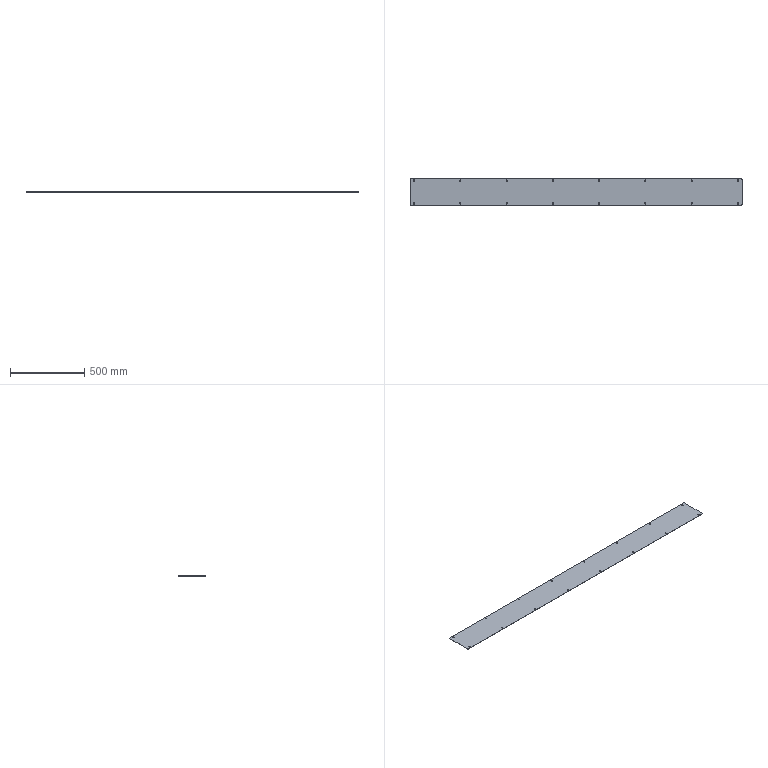Part | SolidWorks | features Fillet 1, FlatPattern 1, ICE 1, LPattern 1, SMBaseFlange 1, SheetMetal 1 | 1 solid | 74 faces | box 2232 x 176 x 1.5 mm | volume 587982 mm3 | plane 38 | cylinder 36 | commonest cylinder face diameters 6 x36